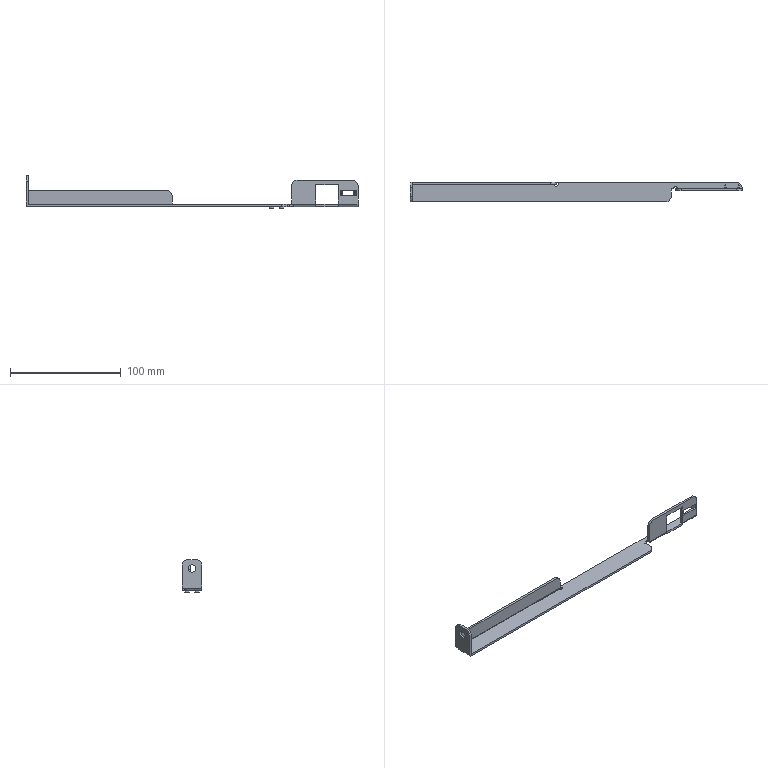Part | STEP file | Lower pull rod (lower door)_6 | 1 solid | 84 faces | box 300 x 18 x 29.5 mm | volume 15254 mm3 | plane 48 | cylinder 28 | spline 8 | commonest cylinder face diameters 4 x7 10 x7 0.6 x4 4.6 x4 4.62 x2 7 x2